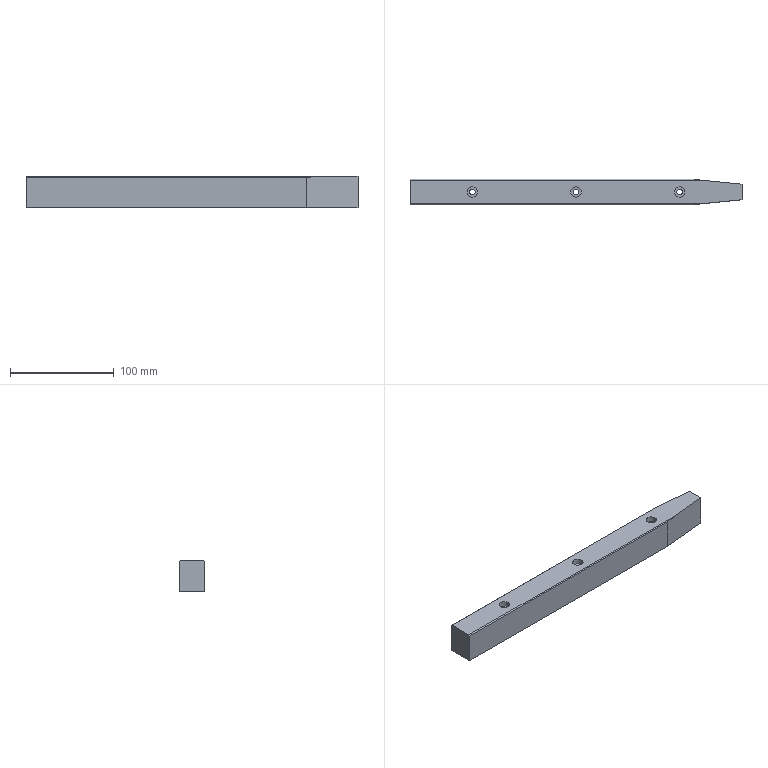Part | STEP file | 1 solid | 25 faces | box 320 x 25 x 30 mm | volume 229201 mm3 | plane 13 | cylinder 12 | commonest cylinder face diameters 5.5 x6 10 x6